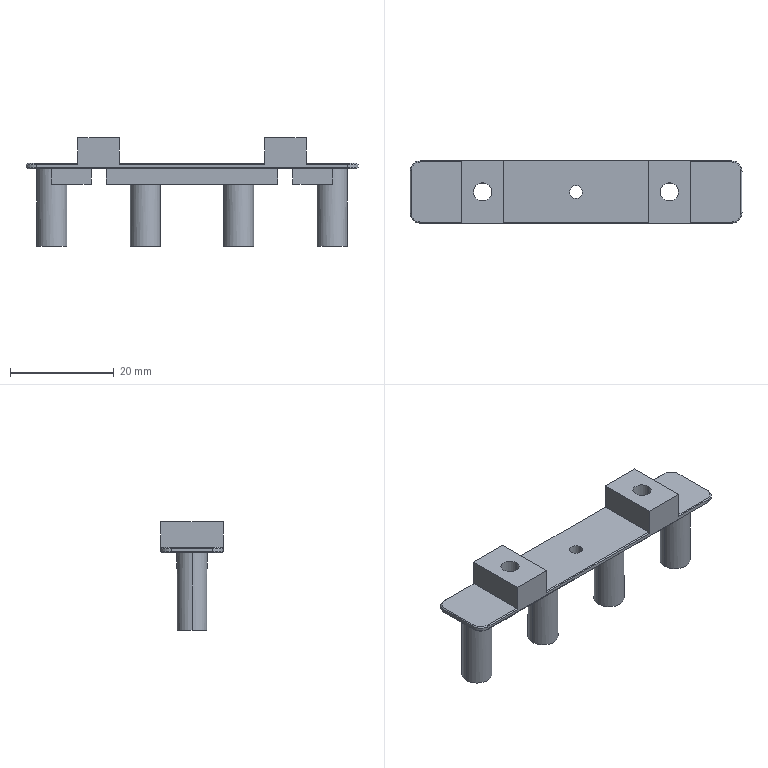Part | 1 solid | 82 faces | box 64 x 12 x 21 mm | volume 3395 mm3 | plane 44 | cylinder 30 | cone 8 | commonest cylinder face diameters 5.1 x8 5.8 x8 3.5 x4 4 x4 6.5 x4 2.5 x2